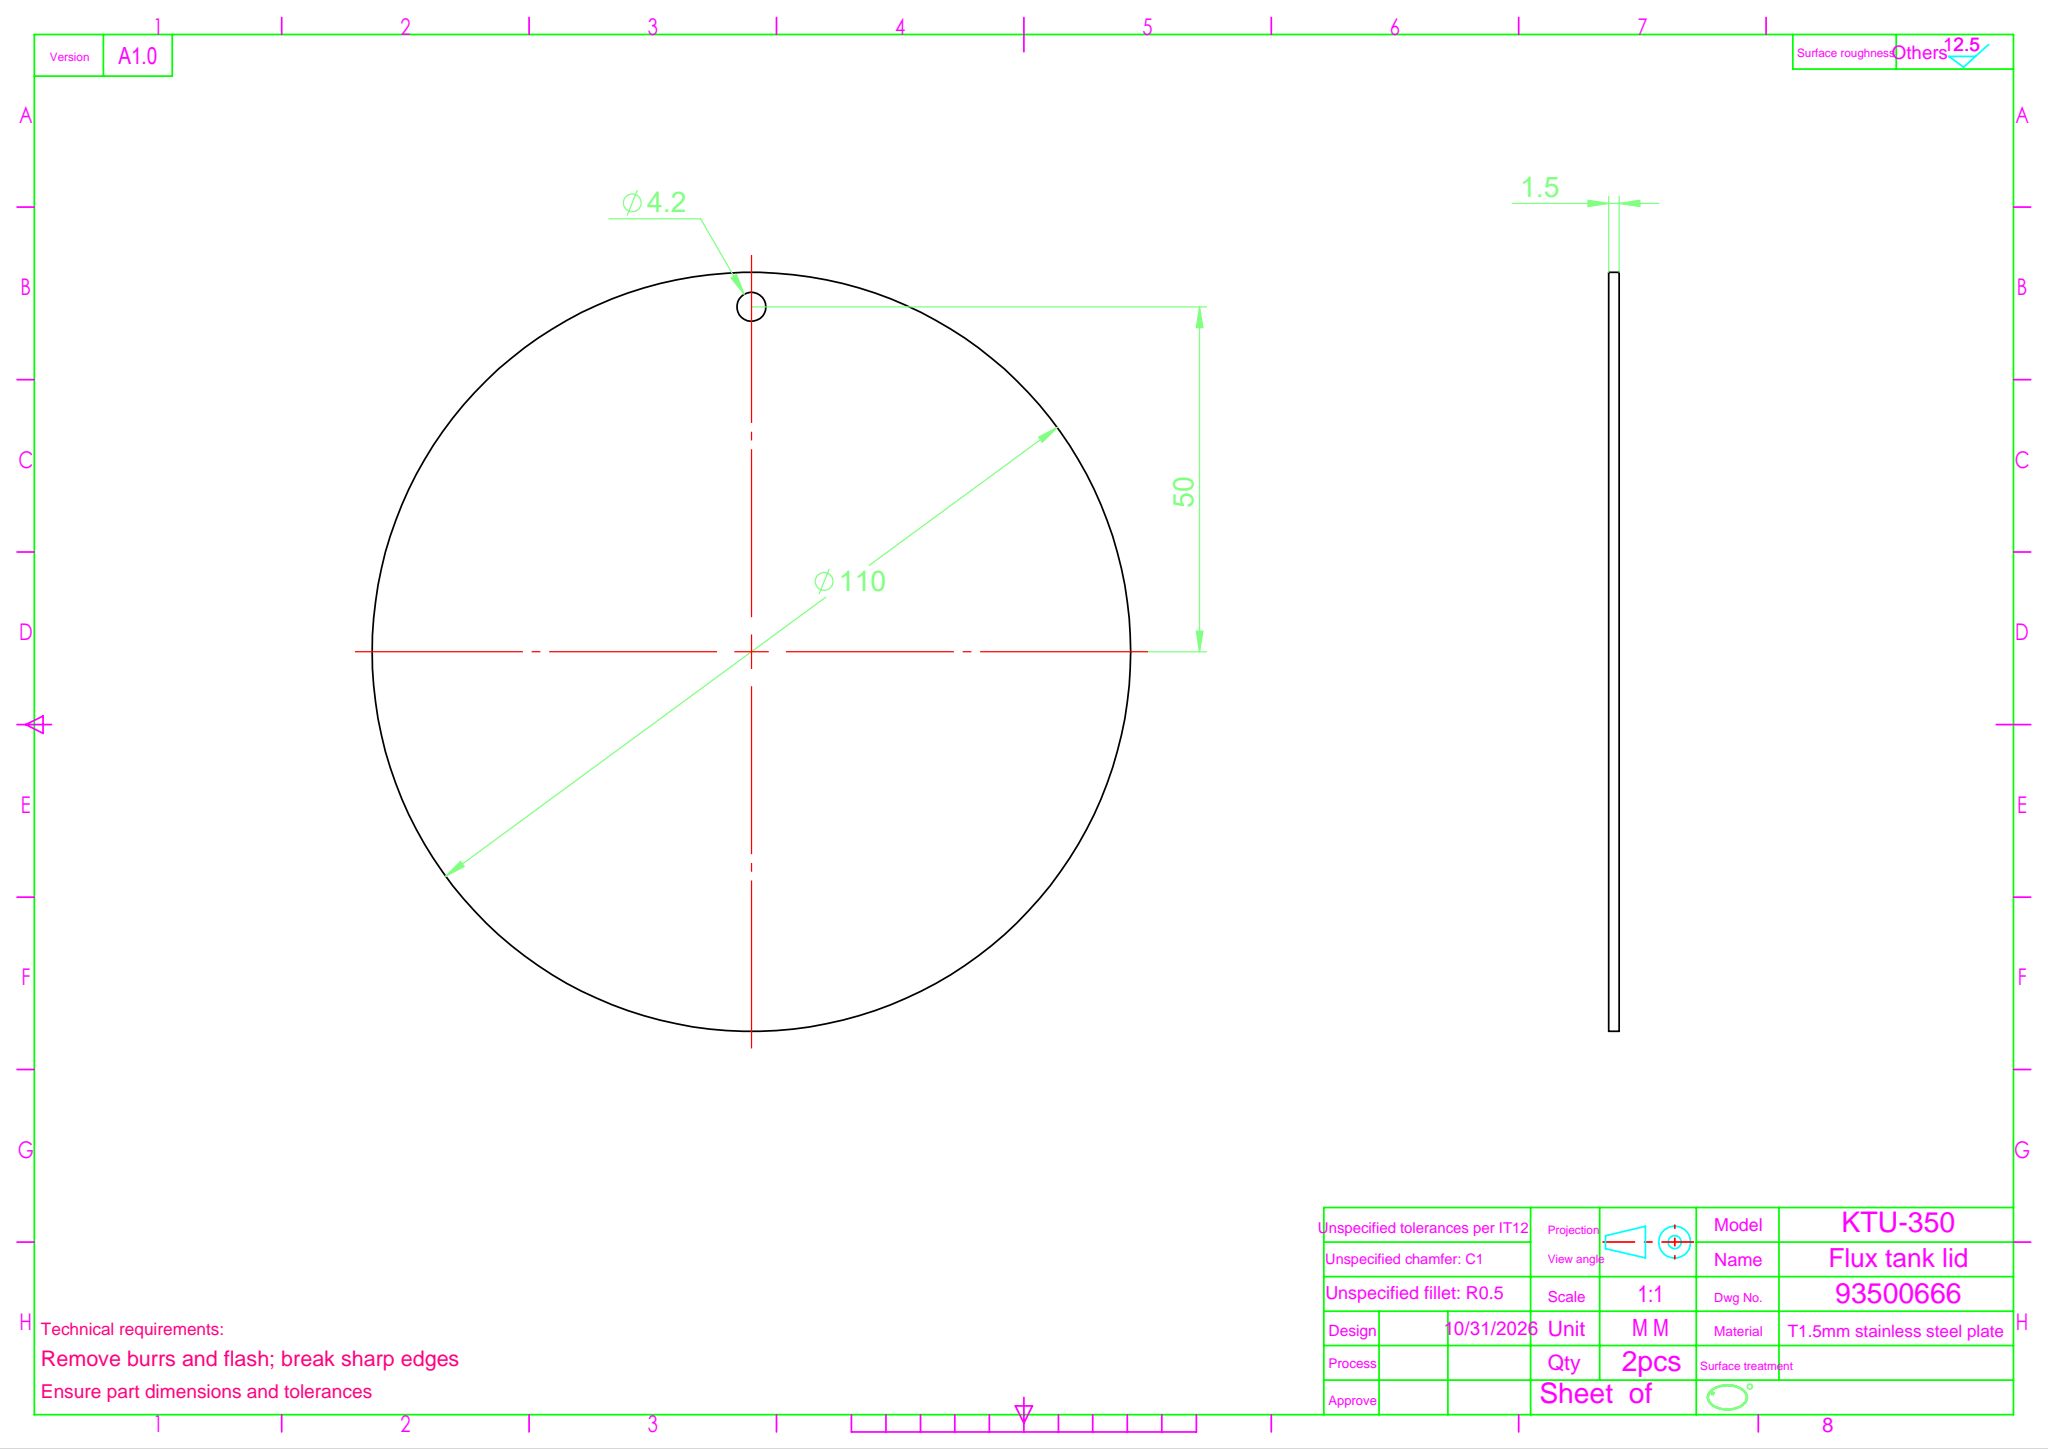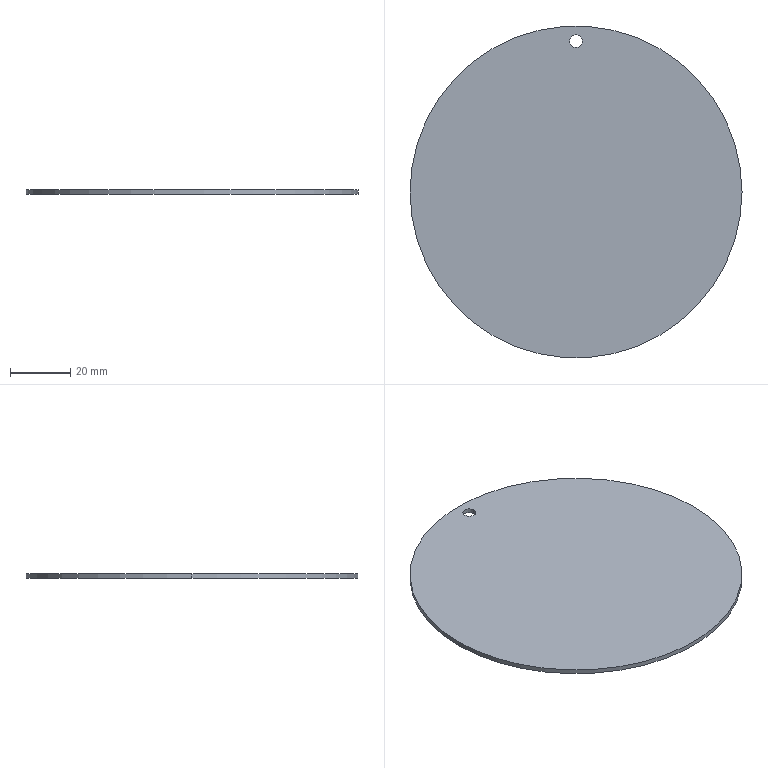Part | SolidWorks | features Extrusion 1, ICE 1 | 1 solid | 6 faces | box 110 x 110 x 1.5 mm | volume 14234 mm3 | cylinder 4 | plane 2 | commonest cylinder face diameters 4.2 x2 110 x2
STEP:
#1=CARTESIAN_POINT('',(-2.1,50.,0.));
#2=VERTEX_POINT('',#1);
#3=CARTESIAN_POINT('',(2.1,50.,0.));
#4=VERTEX_POINT('',#3);
#5=CARTESIAN_POINT('',(0.,50.,0.));
#6=DIRECTION('',(0.,0.,1.));
#7=DIRECTION('',(1.,0.,0.));
#8=AXIS2_PLACEMENT_3D('',#5,#6,#7);
#9=CIRCLE('',#8,2.1);
#10=EDGE_CURVE('',#2,#4,#9,.T.);
#11=ORIENTED_EDGE('',*,*,#10,.F.);
#12=CARTESIAN_POINT('',(-2.1,50.,1.5));
#13=VERTEX_POINT('',#12);
#14=CARTESIAN_POINT('',(-2.1,50.,0.));
#15=DIRECTION('',(0.,0.,1.));
#16=VECTOR('',#15,1000.);
#17=LINE('',#14,#16);
#18=EDGE_CURVE('',#2,#13,#17,.T.);
#19=ORIENTED_EDGE('',*,*,#18,.T.);
#20=CARTESIAN_POINT('',(2.1,50.,1.5));
#21=VERTEX_POINT('',#20);
#22=CARTESIAN_POINT('',(0.,50.,1.5));
#23=DIRECTION('',(0.,0.,1.));
#24=DIRECTION('',(1.,0.,0.));
#25=AXIS2_PLACEMENT_3D('',#22,#23,#24);
#26=CIRCLE('',#25,2.1);
#27=EDGE_CURVE('',#13,#21,#26,.T.);
#28=ORIENTED_EDGE('',*,*,#27,.T.);
#29=CARTESIAN_POINT('',(2.1,50.,0.));
#30=DIRECTION('',(0.,0.,1.));
#31=VECTOR('',#30,1000.);
#32=LINE('',#29,#31);
#33=EDGE_CURVE('',#4,#21,#32,.T.);
#34=ORIENTED_EDGE('',*,*,#33,.F.);
#35=EDGE_LOOP('',(#11,#19,#28,#34));
#36=FACE_OUTER_BOUND('',#35,.T.);
#37=CARTESIAN_POINT('',(0.,50.,0.));
#38=DIRECTION('',(0.,0.,1.));
#39=DIRECTION('',(1.,0.,0.));
#40=AXIS2_PLACEMENT_3D('',#37,#38,#39);
#41=CYLINDRICAL_SURFACE('',#40,2.1);
#42=ADVANCED_FACE('',(#36),#41,.F.);
#43=CARTESIAN_POINT('',(55.,0.,1.5));
#44=VERTEX_POINT('',#43);
#45=CARTESIAN_POINT('',(-55.,0.,1.5));
#46=VERTEX_POINT('',#45);
#47=CARTESIAN_POINT('',(0.,0.,1.5));
#48=DIRECTION('',(0.,0.,1.));
#49=DIRECTION('',(1.,0.,0.));
#50=AXIS2_PLACEMENT_3D('',#47,#48,#49);
#51=CIRCLE('',#50,55.);
#52=EDGE_CURVE('',#44,#46,#51,.T.);
#53=ORIENTED_EDGE('',*,*,#52,.F.);
#54=CARTESIAN_POINT('',(55.,0.,0.));
#55=VERTEX_POINT('',#54);
#56=CARTESIAN_POINT('',(55.,0.,1.5));
#57=DIRECTION('',(0.,0.,-1.));
#58=VECTOR('',#57,1000.);
#59=LINE('',#56,#58);
#60=EDGE_CURVE('',#44,#55,#59,.T.);
#61=ORIENTED_EDGE('',*,*,#60,.T.);
#62=CARTESIAN_POINT('',(-55.,0.,0.));
#63=VERTEX_POINT('',#62);
#64=CARTESIAN_POINT('',(0.,0.,0.));
#65=DIRECTION('',(0.,0.,1.));
#66=DIRECTION('',(1.,0.,0.));
#67=AXIS2_PLACEMENT_3D('',#64,#65,#66);
#68=CIRCLE('',#67,55.);
#69=EDGE_CURVE('',#55,#63,#68,.T.);
#70=ORIENTED_EDGE('',*,*,#69,.T.);
#71=CARTESIAN_POINT('',(-55.,0.,1.5));
#72=DIRECTION('',(0.,0.,-1.));
#73=VECTOR('',#72,1000.);
#74=LINE('',#71,#73);
#75=EDGE_CURVE('',#46,#63,#74,.T.);
#76=ORIENTED_EDGE('',*,*,#75,.F.);
#77=EDGE_LOOP('',(#53,#61,#70,#76));
#78=FACE_OUTER_BOUND('',#77,.T.);
#79=CARTESIAN_POINT('',(0.,0.,1.5));
#80=DIRECTION('',(0.,0.,-1.));
#81=DIRECTION('',(-1.,0.,0.));
#82=AXIS2_PLACEMENT_3D('',#79,#80,#81);
#83=CYLINDRICAL_SURFACE('',#82,55.);
#84=ADVANCED_FACE('',(#78),#83,.T.);
#85=ORIENTED_EDGE('',*,*,#60,.F.);
#86=CARTESIAN_POINT('',(0.,0.,1.5));
#87=DIRECTION('',(0.,0.,1.));
#88=DIRECTION('',(1.,0.,0.));
#89=AXIS2_PLACEMENT_3D('',#86,#87,#88);
#90=CIRCLE('',#89,55.);
#91=EDGE_CURVE('',#46,#44,#90,.T.);
#92=ORIENTED_EDGE('',*,*,#91,.F.);
#93=ORIENTED_EDGE('',*,*,#75,.T.);
#94=CARTESIAN_POINT('',(0.,0.,0.));
#95=DIRECTION('',(0.,0.,1.));
#96=DIRECTION('',(1.,0.,0.));
#97=AXIS2_PLACEMENT_3D('',#94,#95,#96);
#98=CIRCLE('',#97,55.);
#99=EDGE_CURVE('',#63,#55,#98,.T.);
#100=ORIENTED_EDGE('',*,*,#99,.T.);
#101=EDGE_LOOP('',(#85,#92,#93,#100));
#102=FACE_OUTER_BOUND('',#101,.T.);
#103=CARTESIAN_POINT('',(0.,0.,1.5));
#104=DIRECTION('',(0.,0.,-1.));
#105=DIRECTION('',(-1.,0.,0.));
#106=AXIS2_PLACEMENT_3D('',#103,#104,#105);
#107=CYLINDRICAL_SURFACE('',#106,55.);
#108=ADVANCED_FACE('',(#102),#107,.T.);
#109=CARTESIAN_POINT('',(0.,50.,1.5));
#110=DIRECTION('',(0.,0.,1.));
#111=DIRECTION('',(1.,0.,0.));
#112=AXIS2_PLACEMENT_3D('',#109,#110,#111);
#113=CIRCLE('',#112,2.1);
#114=EDGE_CURVE('',#21,#13,#113,.T.);
#115=ORIENTED_EDGE('',*,*,#114,.F.);
#116=ORIENTED_EDGE('',*,*,#27,.F.);
#117=EDGE_LOOP('',(#115,#116));
#118=FACE_BOUND('',#117,.T.);
#119=ORIENTED_EDGE('',*,*,#91,.T.);
#120=ORIENTED_EDGE('',*,*,#52,.T.);
#121=EDGE_LOOP('',(#119,#120));
#122=FACE_OUTER_BOUND('',#121,.T.);
#123=CARTESIAN_POINT('',(0.,0.,1.5));
#124=DIRECTION('',(0.,0.,1.));
#125=DIRECTION('',(1.,0.,0.));
#126=AXIS2_PLACEMENT_3D('',#123,#124,#125);
#127=PLANE('',#126);
#128=ADVANCED_FACE('',(#118,#122),#127,.T.);
#129=CARTESIAN_POINT('',(0.,50.,0.));
#130=DIRECTION('',(0.,0.,1.));
#131=DIRECTION('',(1.,0.,0.));
#132=AXIS2_PLACEMENT_3D('',#129,#130,#131);
#133=CIRCLE('',#132,2.1);
#134=EDGE_CURVE('',#4,#2,#133,.T.);
#135=ORIENTED_EDGE('',*,*,#134,.T.);
#136=ORIENTED_EDGE('',*,*,#10,.T.);
#137=EDGE_LOOP('',(#135,#136));
#138=FACE_BOUND('',#137,.T.);
#139=ORIENTED_EDGE('',*,*,#99,.F.);
#140=ORIENTED_EDGE('',*,*,#69,.F.);
#141=EDGE_LOOP('',(#139,#140));
#142=FACE_OUTER_BOUND('',#141,.T.);
#143=CARTESIAN_POINT('',(0.,0.,0.));
#144=DIRECTION('',(0.,0.,1.));
#145=DIRECTION('',(1.,0.,0.));
#146=AXIS2_PLACEMENT_3D('',#143,#144,#145);
#147=PLANE('',#146);
#148=ADVANCED_FACE('',(#138,#142),#147,.F.);
#149=ORIENTED_EDGE('',*,*,#18,.F.);
#150=ORIENTED_EDGE('',*,*,#134,.F.);
#151=ORIENTED_EDGE('',*,*,#33,.T.);
#152=ORIENTED_EDGE('',*,*,#114,.T.);
#153=EDGE_LOOP('',(#149,#150,#151,#152));
#154=FACE_OUTER_BOUND('',#153,.T.);
#155=CARTESIAN_POINT('',(0.,50.,0.));
#156=DIRECTION('',(0.,0.,1.));
#157=DIRECTION('',(1.,0.,0.));
#158=AXIS2_PLACEMENT_3D('',#155,#156,#157);
#159=CYLINDRICAL_SURFACE('',#158,2.1);
#160=ADVANCED_FACE('',(#154),#159,.F.);
#161=CLOSED_SHELL('',(#42,#84,#108,#128,#148,#160));
#162=MANIFOLD_SOLID_BREP('',#161);
#163=CARTESIAN_POINT('',(0.,0.,0.));
#164=DIRECTION('',(0.,0.,1.));
#165=DIRECTION('',(1.,0.,0.));
#166=AXIS2_PLACEMENT_3D('',#163,#164,#165);
#167=(LENGTH_UNIT()NAMED_UNIT(*)SI_UNIT(.MILLI.,.METRE.));
#168=UNCERTAINTY_MEASURE_WITH_UNIT(LENGTH_MEASURE(0.00001),#167,'','');
#169=(NAMED_UNIT(*)PLANE_ANGLE_UNIT()SI_UNIT($,.RADIAN.));
#170=(NAMED_UNIT(*)SI_UNIT($,.STERADIAN.)SOLID_ANGLE_UNIT());
#171=(GEOMETRIC_REPRESENTATION_CONTEXT(3)GLOBAL_UNCERTAINTY_ASSIGNED_CONTEXT((#168))GLOBAL_UNIT_ASSIGNED_CONTEXT((#167,#169,#170))REPRESENTATION_CONTEXT('',''));
#172=ADVANCED_BREP_SHAPE_REPRESENTATION('',(#162,#166),#171);